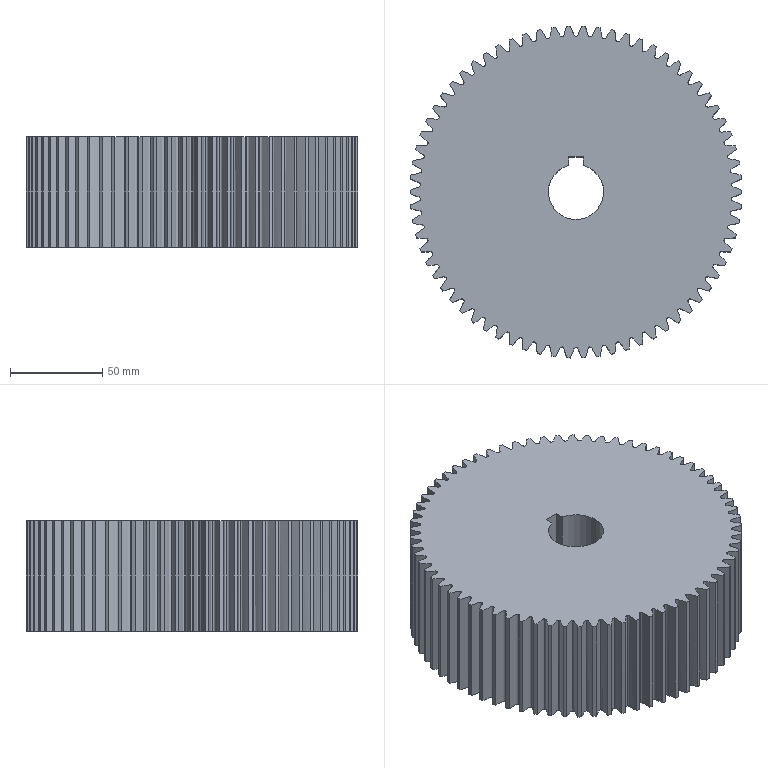Part | SolidWorks | features ICE 3, CirPattern 1, Extrusion 1, RefAxis 1 | 1 solid | 289 faces | box 180 x 179.897 x 60 mm | volume 1397109 mm3 | cylinder 144 | spline 140 | plane 5 | commonest cylinder face diameters 180 x71 168.749 x70 30 x3